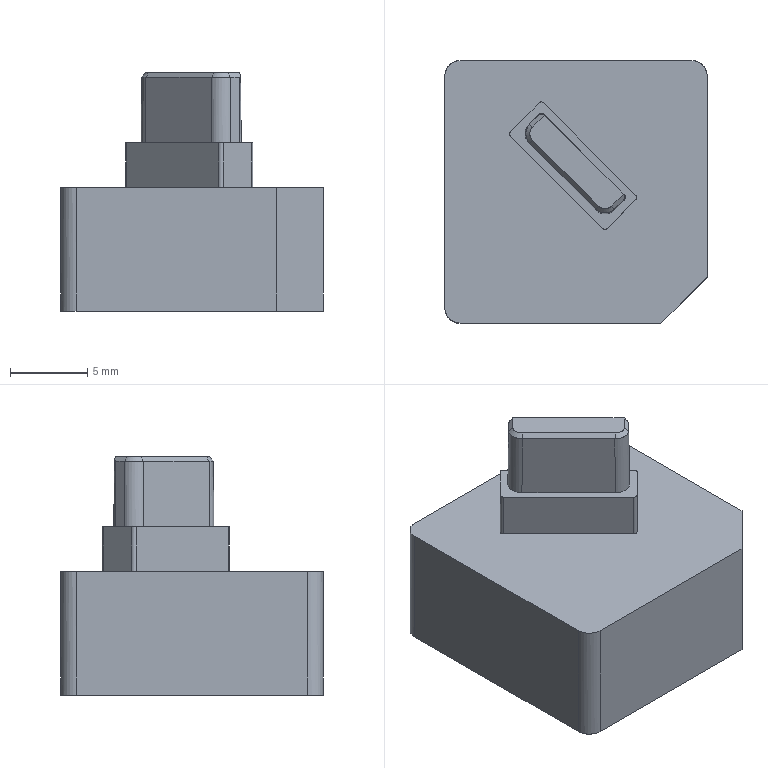CAM job | PowerMill | 3-axis milling, other | part box 17 x 17 x 15.424 mm
Tools:
number,name,type,diameter,tip_radius,length,cutting_length,overhang,flutes,holder,toolpaths_using
1,D10C_1_1,end_mill,10.0,0.0,60.0,,15.88,1,D42L35,6
3,D10_1_1,end_mill,10.0,0.0,60.0,,15.6,1,D42L35,8
14,D4_1_1,end_mill,4.0,0.0,30.0,,7.6,1,D42L35,2
13,Text_D4_1_1,taper_spherical,4.0,0.3,60.0,,7.68,1,D42L35,2
14,D4_2_1,end_mill,4.0,0.0,30.0,,7.44,1,D42L35,2
Operations:
program,toolpath,strategy,tool,tool_number,tool_diameter,tip_radius,flutes,spindle_rpm,feed_cut,surface_speed_m_min_computed,feed_per_tooth_computed,tolerance,thickness,stepover,stepdown,cut_length,cut_time_min,total_time_min,workplane
04-C01-4-F,精公开粗01-扫面平行-D10C,raster_area_clear,D10C_1_1,1,10.0,0.0,1.0,8000.0,10000.0,251.33,1.25,0.03,0.28,6.0,1.0,135.36,0.013,0.0178,
04-C01-4-F,精公开粗01-外形偏置-D10C,offset_area_clear,D10C_1_1,1,10.0,0.0,1.0,8000.0,10000.0,251.33,1.25,0.03,0.28,6.0,1.0,3105.167,0.31,0.3614,
04-C01-4-F,精公开粗01-基准台等高-D10C,constantz,D10C_1_1,1,10.0,0.0,1.0,8000.0,10000.0,251.33,1.25,0.03,0.07,5.0,0.4,2129.063,0.213,0.2214,
04-C01-4-F,精公基准台01-平坦面平行-D10,raster_area_clear,D10_1_1,3,10.0,0.0,1.0,8500.0,600.0,267.04,0.0706,0.005,0.38,5.0,1.0,104.613,0.174,0.2251,
04-C01-4-F,精公基准台01-基准面偏置-D10,offset_area_clear,D10_1_1,3,10.0,0.0,1.0,8500.0,600.0,267.04,0.0706,0.005,0.38,5.0,1.0,79.027,0.132,0.1491,
04-C01-4-F,精公基准台01-外形侧光-D10,profile_area_clear,D10_1_1,3,10.0,0.0,1.0,8500.0,600.0,267.04,0.0706,0.005,-0.07,0.08,1.0,109.346,0.182,0.2014,
04-C01-4-F,精公基准台01-基准台侧光-D10,profile_area_clear,D10_1_1,3,10.0,0.0,1.0,8500.0,600.0,267.04,0.0706,0.005,0.0,0.08,1.0,193.234,0.322,0.3848,
04-C01-4-F,精公精光01-等高-D4,constantz,D4_1_1,14,4.0,0.0,1.0,18000.0,2000.0,226.19,0.1111,0.005,-0.075,5.0,0.02,5056.987,2.529,2.789,
04-C01-4-F,精公精光01-平坦面平行-D4,raster_area_clear,D4_1_1,14,4.0,0.0,1.0,18000.0,600.0,226.19,0.0333,0.005,0.375,2.0,1.0,38.41,0.064,0.0739,
04-C01-4-F,精公刻字01-刻字-Text_D4,pattern,Text_D4_1_1,13,4.0,0.3,1.0,15000.0,1000.0,188.5,0.0667,0.005,0.0,5.0,1.0,23.664,0.024,0.0392,
04-C01-4-R,粗公开粗01-扫面平行-D10C,raster_area_clear,D10C_1_1,1,10.0,0.0,1.0,8000.0,10000.0,251.33,1.25,0.03,0.15,6.0,1.0,133.8,0.013,0.0185,
04-C01-4-R,粗公开粗01-外形偏置-D10C,offset_area_clear,D10C_1_1,1,10.0,0.0,1.0,8000.0,10000.0,251.33,1.25,0.03,0.15,6.0,1.0,2912.645,0.291,0.3399,
04-C01-4-R,粗公开粗01-基准台等高-D10C,constantz,D10C_1_1,1,10.0,0.0,1.0,8000.0,10000.0,251.33,1.25,0.03,0.07,5.0,0.4,2129.063,0.213,0.2214,
04-C01-4-R,粗公基准台01-平坦面平行-D10,raster_area_clear,D10_1_1,3,10.0,0.0,1.0,8500.0,600.0,267.04,0.0706,0.01,0.25,5.0,1.0,96.582,0.161,0.2114,
04-C01-4-R,粗公基准台01-基准面偏置-D10,offset_area_clear,D10_1_1,3,10.0,0.0,1.0,8500.0,600.0,267.04,0.0706,0.01,0.25,5.0,1.0,77.836,0.13,0.1471,
04-C01-4-R,粗公基准台01-外形侧光-D10,profile_area_clear,D10_1_1,3,10.0,0.0,1.0,8500.0,600.0,267.04,0.0706,0.01,-0.2,0.08,1.0,107.699,0.179,0.1987,
04-C01-4-R,粗公基准台01-基准台侧光-D10,profile_area_clear,D10_1_1,3,10.0,0.0,1.0,8500.0,600.0,267.04,0.0706,0.01,0.0,0.08,1.0,193.218,0.322,0.3848,
04-C01-4-R,粗公精光01-等高-D4,constantz,D4_2_1,14,4.0,0.0,1.0,18000.0,2000.0,226.19,0.1111,0.01,-0.205,5.0,0.02,4158.122,2.079,2.3,
04-C01-4-R,粗公精光01-平坦面平行-D4,raster_area_clear,D4_2_1,14,4.0,0.0,1.0,18000.0,600.0,226.19,0.0333,0.01,0.245,2.0,1.0,37.605,0.063,0.0727,
04-C01-4-R,粗公刻字01-刻字-Text_D4,pattern,Text_D4_1_1,13,4.0,0.3,1.0,15000.0,1000.0,188.5,0.0667,0.01,0.0,5.0,1.0,23.45,0.023,0.0382,